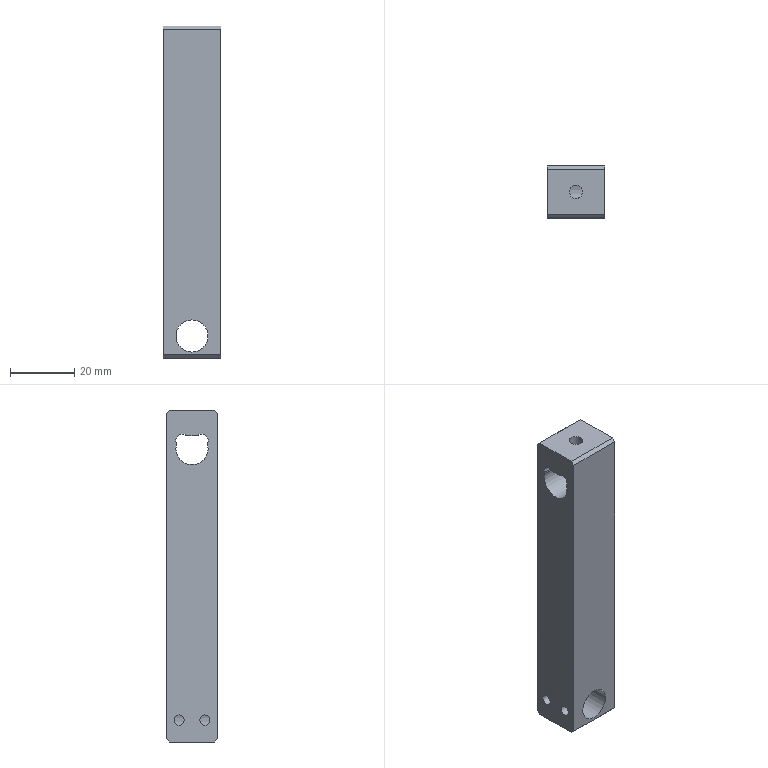CAM job | NX | 3+2 milling, drilling | part box 18 x 16 x 103.264 mm | stock box 20 x 20 x 108.264 mm
Tools:
number,name,description,diameter,corner_radius,flute_length,length,flutes
4,D4,平底铣刀-粗,4.0,0.0,25.0,75.0,2
6,D6,平底铣刀-粗,6.0,0.0,25.0,75.0,2
9,D10,平底铣刀-粗,10.0,0.0,35.0,75.0,2
11,D4-J,平底铣刀-精,4.0,0.0,50.0,75.0,2
7,D6-J,平底铣刀-精,6.0,0.0,25.0,75.0,2
10,D10-J,平底铣刀-精,10.0,0.0,35.0,75.0,2
1,D80R0.8飞刀,圆鼻刀-粗,80.0,0.8,50.0,75.0,2
1,D80R0.8飞刀-J,圆鼻刀-精,80.0,0.8,50.0,75.0,2
2,D6倒角刀,倒角刀,6.0,0.0,3.0,25.0,2
21,M4X0.7,丝锥,3.3,0.0,35.0,50.0,2
13,ZT3.3,钻头,3.3,0.0,35.0,50.0,2
16,ZT6.8,钻头,6.8,0.0,35.0,50.0,2
17,ZT9.5,钻头,9.5,0.0,35.0,50.0,2
Operations:
program,operation,operation_type,tool,method,geometry_group,spindle_rpm,surface_speed,feed_per_tooth,feed_cut,feed_plunge,cut_length_mm,path_length_mm,cut_time_min,machine_time_min
C,打点-深0.8_2,Operation,D6倒角刀,NONE,W-C,8000.0,150.796,0.0312,500.0,90.0,3.6,56.262,0.0072,0.0125
C,打点-深0.8_2_COPY,Operation,D6倒角刀,NONE,W-C,8000.0,150.796,0.0312,500.0,90.0,1.8,43.6,0.0036,0.0078
C,通孔-M4螺纹底孔,Operation,ZT3.3,NONE,W-C,3000.0,30.159,0.05,300.0,90.0,22.0,93.062,0.0733,0.0804
C,通孔-M4螺纹底孔_COPY,Operation,ZT6.8,NONE,W-C,2000.0,42.726,0.075,300.0,90.0,23.0,86.0,0.0767,0.083
C,底壁铣螺旋开粗-中_COPY,VolumeBased25DMillingOperation,D4,分层开粗-切深K-步距G,W-C,8000.0,100.528,0.125,2000.0,100.0,1292.207,1348.707,0.6461,0.6518
C,钻倒角_1,Operation,D6倒角刀,METHOD,W-C,8000.0,150.796,0.0312,500.0,0.0,10.3,72.144,0.0206,0.0268
C,C0.3封闭铣廓倒角6X45L_COPY,PlanarMilling,D6倒角刀,爬面_倒角-切深0-步距G,W-C,7000.0,131.0,0.1071,1500.0,100.0,42.301,78.301,0.0282,0.0318
C,通孔-攻牙M4,Operation,M4X0.7,METHOD,W-C,600.0,6.22,0.0006,0.7,90.0,16.0,81.062,22.857,22.864
C,底壁铣螺旋精光-中_COPY,VolumeBased25DMillingOperation,D4-J,螺旋精光-切深K-步距G,W-C,8000.0,100.528,0.05,800.0,100.0,242.73,299.73,0.3034,0.3091
B,底壁铣飞面一刀开粗_COPY,VolumeBased25DMillingOperation,D80R0.8飞刀,分层开粗-切深K-步距G,W-B,5000.0,1256.637,0.3,3000.0,100.0,1691.666,3311.663,0.5639,0.7259
B,底壁铣飞面一刀精光_COPY,VolumeBased25DMillingOperation,D80R0.8飞刀-J,侧刃精光-切深K-步距G,W-B,5000.0,1256.637,0.1,1000.0,100.0,211.262,247.262,0.2113,0.2149
B,平面去毛刺6X45L_COPY,SurfaceContour,D6倒角刀,爬面_倒角-切深0-步距G,W-B,6500.0,122.519,0.1154,1500.0,100.0,239.983,334.868,0.16,0.1695
B,底壁铣倒角_COPY_1,VolumeBased25DMillingOperation,D6倒角刀,爬面_倒角-切深0-步距G,W-B,6500.0,122.519,0.1154,1500.0,100.0,108.422,342.307,0.0723,0.0957
A,顶面,FaceMilling,D80R0.8飞刀,侧刃精光-切深K-步距G,W-A,5000.0,1256.637,0.1,1000.0,100.0,197.264,233.264,0.1973,0.2009
A,外形粗_2,VolumeBased25DMillingOperation,D10,METHOD,W-A,8000.0,251.327,0.3125,5000.0,80.0,6316.696,6371.496,1.263,1.269
A,打点-深0.8,Operation,D6倒角刀,NONE,W-A,8000.0,150.796,0.0312,500.0,90.0,1.8,43.6,0.0036,0.0078
A,通孔-精孔10.0预钻,Operation,ZT9.5,NONE,W-A,1000.0,31.102,0.15,300.0,90.0,22.854,85.708,0.0762,0.0825
A,铣孔开粗D6_1,CylinderMilling,D6,NONE,W-A,8000.0,150.796,0.0625,1000.0,100.0,433.072,489.072,0.4331,0.4387
A,仅选体,SurfaceContour,D6倒角刀,METHOD,W-A,8000.0,150.796,0.1875,3000.0,100.0,222.155,310.831,0.0741,0.0829
A,铣倒角_1,PlanarMilling,D6倒角刀,METHOD,W-A,8000.0,150.796,0.0312,500.0,100.0,37.443,78.442,0.0749,0.079
A,底壁铣倒角_COPY,VolumeBased25DMillingOperation,D6倒角刀,爬面_倒角-切深0-步距G,W-A,6500.0,122.519,0.1154,1500.0,100.0,53.601,239.081,0.0357,0.0543
A,铣孔精光D6-J_1,CylinderMilling,D6-J,精光步距切深关,W-A,8000.0,150.796,0.0312,500.0,100.0,236.574,292.574,0.4731,0.4787
A,外形半精_2,VolumeBased25DMillingOperation,D10-J,METHOD,W-A,8000.0,251.327,0.0625,1000.0,100.0,278.903,350.503,0.2789,0.2861